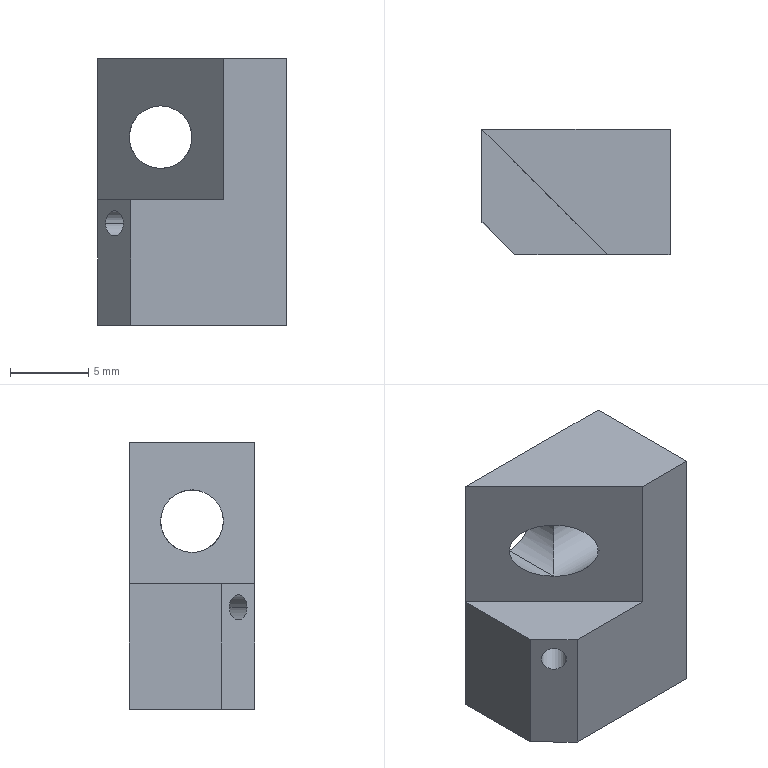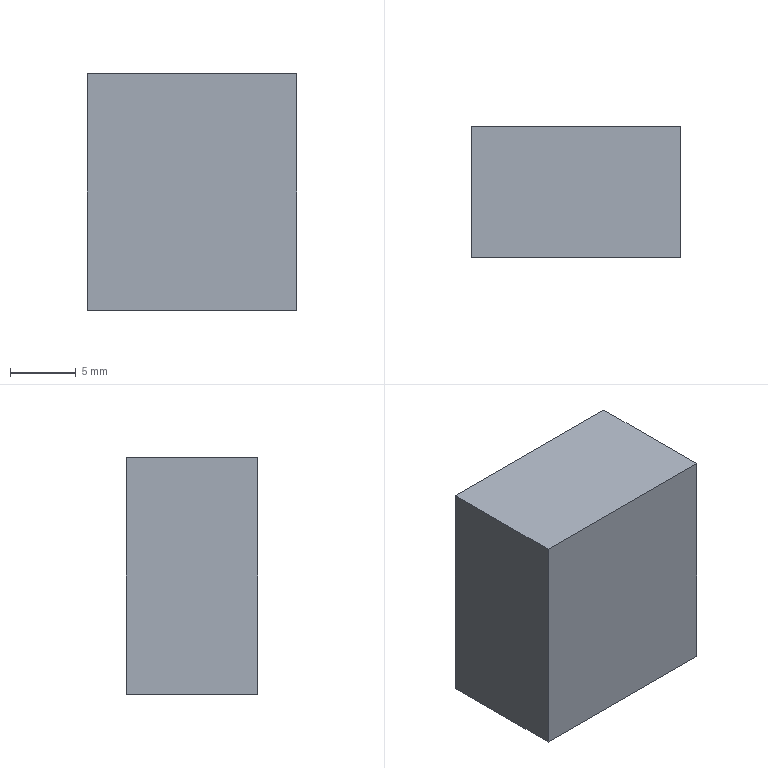CAM job | NX | 3-axis milling, drilling | part box 12 x 8 x 17 mm | stock box 16 x 10 x 18 mm
Tools:
number,name,description,diameter,corner_radius,flute_length,length,flutes
9,D10JING,Milling Tool-5 Parameters,10.0,0.0,50.0,75.0,2
6,D6,Milling Tool-5 Parameters,6.0,0.0,50.0,75.0,2
7,D6A45,Milling Tool-5 Parameters,6.0,0.0,50.0,75.0,2
14,1.6ZT,Drilling Tool,1.6,0.0,35.0,50.0,2
1,D1.,Milling Tool-5 Parameters,1.0,0.0,50.0,75.0,2
Operations:
program,operation,operation_type,tool,method,geometry_group,spindle_rpm,surface_speed,feed_per_tooth,feed_cut,feed_plunge,cut_length_mm,path_length_mm,cut_time_min,machine_time_min
1,FLOOR_WALL,VolumeBased25DMillingOperation,D10JING,METHOD,A,9500.0,298.0,0.0658,1250.0,100.0,95.997,149.997,0.0768,0.0822
1,ZLEVEL_PROFILE,ZLevelMilling,D6,METHOD,A,9500.0,298.0,0.1316,2500.0,1000.0,3372.909,3446.759,1.37,1.377
1,FLOOR_WALL_1,VolumeBased25DMillingOperation,D6,METHOD,A,9500.0,298.0,0.1316,2500.0,1000.0,1070.071,1226.756,0.4747,0.4903
1,FLOOR_WALL_1_COPY,VolumeBased25DMillingOperation,D6,METHOD,A,9500.0,298.0,0.0632,1200.0,1000.0,57.715,135.715,0.0489,0.0567
1,ZLEVEL_PROFILE_1_COPY,ZLevelMilling,D6A45,METHOD,A,9500.0,179.0,0.0658,1250.0,100.0,48.44,106.439,0.0388,0.0446
1,ZLEVEL_PROFILE_COPY_COPY_COPY_COPY_COPY,ZLevelMilling,D6,METHOD,A,9500.0,89.0,0.0632,1200.0,1000.0,165.194,249.044,0.1382,0.1466
2,DRILLING,Operation,D6A45,METHOD,B,5000.0,94.0,0.025,250.0,0.0,15.6,116.971,0.0624,0.0725
2,DRILLING_COPY_COPY,Operation,1.6ZT,METHOD,B,2000.0,20.0,0.0375,150.0,0.0,30.16,146.09,0.2011,0.2127
2,HOLE_MILLING,CylinderMilling,D1.,METHOD,B,9500.0,29.0,0.0526,1000.0,100.0,284.207,415.005,0.2842,0.2973
2,DRILLING_COPY,Operation,D6A45,METHOD,B,5000.0,94.0,0.025,250.0,0.0,8.2,85.231,0.0328,0.0405
2,刀补1,CylinderMilling,D1.,METHOD,B,9500.0,29.0,0.0447,850.0,100.0,32.493,163.292,0.0382,0.0513